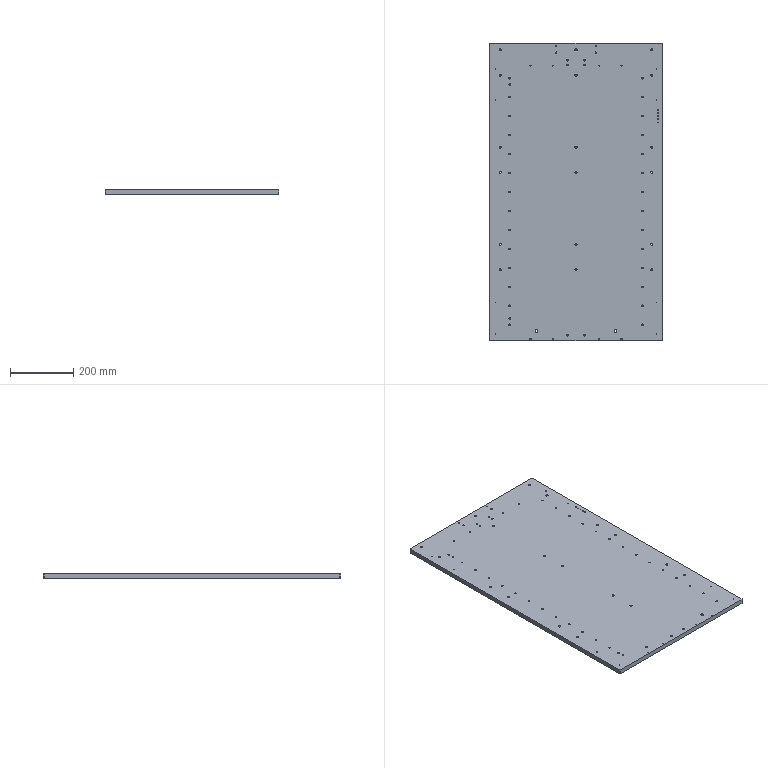Part | NX | 1 solid | 106 faces | box 550 x 940 x 15 mm | volume 7730594 mm3 | cylinder 81 | cone 15 | plane 10 | commonest cylinder face diameters 5 x36 6.8 x18 2.5 x13 3.3 x8 4.2 x4 8.5 x2